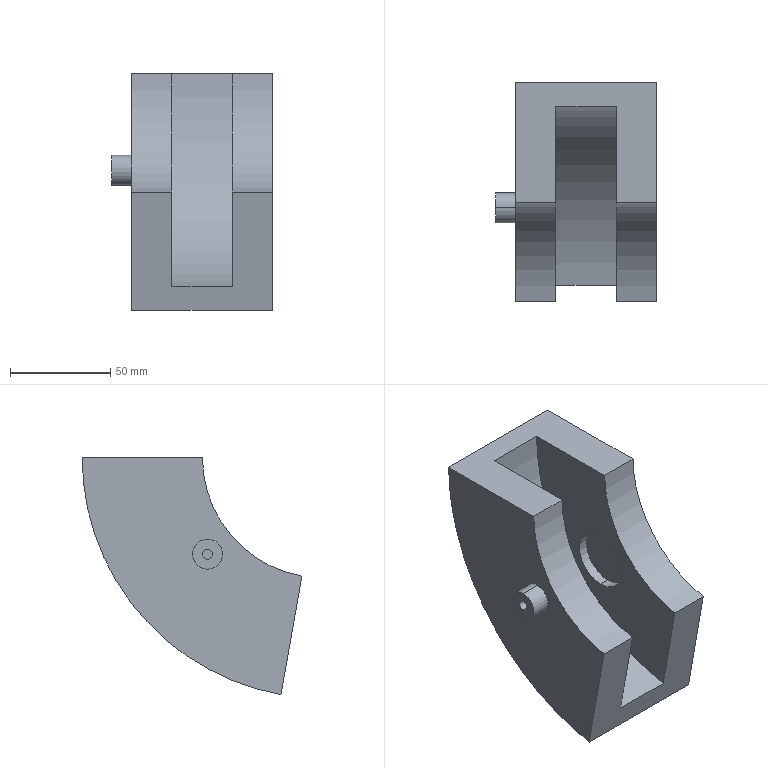Part | SolidWorks | features Cut 1, ICE 1, Revolution 1, Shell 1 | 1 solid | 29 faces | box 80 x 109.581 x 118.177 mm | volume 225708 mm3 | cylinder 16 | plane 13 | commonest cylinder face diameters 30 x4 5 x2 15 x2 120 x2 130 x2 216 x1
STEP:
#1=CARTESIAN_POINT('',(-35.136,61.532,-67.709));
#2=VERTEX_POINT('',#1);
#3=CARTESIAN_POINT('',(-35.136,61.532,-37.709));
#4=VERTEX_POINT('',#3);
#5=CARTESIAN_POINT('',(-35.136,61.532,-52.709));
#6=DIRECTION('',(-1.,0.,0.));
#7=DIRECTION('',(0.,1.,0.));
#8=AXIS2_PLACEMENT_3D('',#5,#6,#7);
#9=CIRCLE('',#8,15.);
#10=EDGE_CURVE('',#2,#4,#9,.T.);
#11=ORIENTED_EDGE('',*,*,#10,.T.);
#12=CARTESIAN_POINT('',(-30.136,61.532,-37.709));
#13=VERTEX_POINT('',#12);
#14=CARTESIAN_POINT('',(-60.137,61.532,-37.709));
#15=DIRECTION('',(1.,0.,0.));
#16=VECTOR('',#15,1000.);
#17=LINE('',#14,#16);
#18=EDGE_CURVE('',#4,#13,#17,.T.);
#19=ORIENTED_EDGE('',*,*,#18,.T.);
#20=CARTESIAN_POINT('',(-30.136,61.532,-67.709));
#21=VERTEX_POINT('',#20);
#22=CARTESIAN_POINT('',(-30.136,61.532,-52.709));
#23=DIRECTION('',(1.,0.,0.));
#24=DIRECTION('',(0.,0.,-1.));
#25=AXIS2_PLACEMENT_3D('',#22,#23,#24);
#26=CIRCLE('',#25,15.);
#27=EDGE_CURVE('',#13,#21,#26,.T.);
#28=ORIENTED_EDGE('',*,*,#27,.T.);
#29=CARTESIAN_POINT('',(-60.137,61.532,-67.709));
#30=DIRECTION('',(1.,0.,0.));
#31=VECTOR('',#30,1000.);
#32=LINE('',#29,#31);
#33=EDGE_CURVE('',#2,#21,#32,.T.);
#34=ORIENTED_EDGE('',*,*,#33,.F.);
#35=EDGE_LOOP('',(#11,#19,#28,#34));
#36=FACE_OUTER_BOUND('',#35,.T.);
#37=CARTESIAN_POINT('',(-60.137,61.532,-52.709));
#38=DIRECTION('',(1.,0.,0.));
#39=DIRECTION('',(0.,0.,-1.));
#40=AXIS2_PLACEMENT_3D('',#37,#38,#39);
#41=CYLINDRICAL_SURFACE('',#40,15.);
#42=ADVANCED_FACE('',(#36),#41,.F.);
#43=CARTESIAN_POINT('',(4.864,61.532,-67.709));
#44=VERTEX_POINT('',#43);
#45=CARTESIAN_POINT('',(4.864,61.532,-37.709));
#46=VERTEX_POINT('',#45);
#47=CARTESIAN_POINT('',(4.864,61.532,-52.709));
#48=DIRECTION('',(-1.,0.,0.));
#49=DIRECTION('',(0.,-1.,0.));
#50=AXIS2_PLACEMENT_3D('',#47,#48,#49);
#51=CIRCLE('',#50,15.);
#52=EDGE_CURVE('',#44,#46,#51,.T.);
#53=ORIENTED_EDGE('',*,*,#52,.F.);
#54=CARTESIAN_POINT('',(-0.1364,61.532,-67.709));
#55=VERTEX_POINT('',#54);
#56=CARTESIAN_POINT('',(19.865,61.532,-67.709));
#57=DIRECTION('',(-1.,0.,0.));
#58=VECTOR('',#57,1000.);
#59=LINE('',#56,#58);
#60=EDGE_CURVE('',#44,#55,#59,.T.);
#61=ORIENTED_EDGE('',*,*,#60,.T.);
#62=CARTESIAN_POINT('',(-0.1364,61.532,-37.709));
#63=VERTEX_POINT('',#62);
#64=CARTESIAN_POINT('',(-0.1364,61.532,-52.709));
#65=DIRECTION('',(-1.,0.,0.));
#66=DIRECTION('',(0.,-1.,0.));
#67=AXIS2_PLACEMENT_3D('',#64,#65,#66);
#68=CIRCLE('',#67,15.);
#69=EDGE_CURVE('',#55,#63,#68,.T.);
#70=ORIENTED_EDGE('',*,*,#69,.T.);
#71=CARTESIAN_POINT('',(19.865,61.532,-37.709));
#72=DIRECTION('',(-1.,0.,0.));
#73=VECTOR('',#72,1000.);
#74=LINE('',#71,#73);
#75=EDGE_CURVE('',#46,#63,#74,.T.);
#76=ORIENTED_EDGE('',*,*,#75,.F.);
#77=EDGE_LOOP('',(#53,#61,#70,#76));
#78=FACE_OUTER_BOUND('',#77,.T.);
#79=CARTESIAN_POINT('',(19.865,61.532,-52.709));
#80=DIRECTION('',(-1.,0.,0.));
#81=DIRECTION('',(0.,0.,1.));
#82=AXIS2_PLACEMENT_3D('',#79,#80,#81);
#83=CYLINDRICAL_SURFACE('',#82,15.);
#84=ADVANCED_FACE('',(#78),#83,.F.);
#85=CARTESIAN_POINT('',(-60.136,56.17,-50.709));
#86=VERTEX_POINT('',#85);
#87=CARTESIAN_POINT('',(-60.136,56.17,-45.709));
#88=VERTEX_POINT('',#87);
#89=CARTESIAN_POINT('',(-60.136,56.17,-48.209));
#90=DIRECTION('',(-1.,0.,0.));
#91=DIRECTION('',(0.,0.,1.));
#92=AXIS2_PLACEMENT_3D('',#89,#90,#91);
#93=CIRCLE('',#92,2.5);
#94=EDGE_CURVE('',#86,#88,#93,.T.);
#95=ORIENTED_EDGE('',*,*,#94,.T.);
#96=CARTESIAN_POINT('',(-45.136,56.17,-45.709));
#97=VERTEX_POINT('',#96);
#98=CARTESIAN_POINT('',(-60.136,56.17,-45.709));
#99=DIRECTION('',(1.,0.,0.));
#100=VECTOR('',#99,1000.);
#101=LINE('',#98,#100);
#102=EDGE_CURVE('',#88,#97,#101,.T.);
#103=ORIENTED_EDGE('',*,*,#102,.T.);
#104=CARTESIAN_POINT('',(-45.136,56.17,-50.709));
#105=VERTEX_POINT('',#104);
#106=CARTESIAN_POINT('',(-45.136,56.17,-48.209));
#107=DIRECTION('',(-1.,0.,0.));
#108=DIRECTION('',(0.,-1.,0.));
#109=AXIS2_PLACEMENT_3D('',#106,#107,#108);
#110=CIRCLE('',#109,2.5);
#111=EDGE_CURVE('',#105,#97,#110,.T.);
#112=ORIENTED_EDGE('',*,*,#111,.F.);
#113=CARTESIAN_POINT('',(-60.136,56.17,-50.709));
#114=DIRECTION('',(1.,0.,0.));
#115=VECTOR('',#114,1000.);
#116=LINE('',#113,#115);
#117=EDGE_CURVE('',#86,#105,#116,.T.);
#118=ORIENTED_EDGE('',*,*,#117,.F.);
#119=EDGE_LOOP('',(#95,#103,#112,#118));
#120=FACE_OUTER_BOUND('',#119,.T.);
#121=CARTESIAN_POINT('',(-60.136,56.17,-48.209));
#122=DIRECTION('',(1.,0.,0.));
#123=DIRECTION('',(0.,0.,-1.));
#124=AXIS2_PLACEMENT_3D('',#121,#122,#123);
#125=CYLINDRICAL_SURFACE('',#124,2.5);
#126=ADVANCED_FACE('',(#120),#125,.F.);
#127=CARTESIAN_POINT('',(-60.136,56.17,-40.709));
#128=VERTEX_POINT('',#127);
#129=CARTESIAN_POINT('',(-60.136,56.17,-55.709));
#130=VERTEX_POINT('',#129);
#131=CARTESIAN_POINT('',(-60.136,56.17,-48.209));
#132=DIRECTION('',(-1.,0.,0.));
#133=DIRECTION('',(0.,0.,1.));
#134=AXIS2_PLACEMENT_3D('',#131,#132,#133);
#135=CIRCLE('',#134,7.5);
#136=EDGE_CURVE('',#128,#130,#135,.T.);
#137=ORIENTED_EDGE('',*,*,#136,.F.);
#138=CARTESIAN_POINT('',(-50.136,56.17,-40.709));
#139=VERTEX_POINT('',#138);
#140=CARTESIAN_POINT('',(-60.136,56.17,-40.709));
#141=DIRECTION('',(1.,0.,0.));
#142=VECTOR('',#141,1000.);
#143=LINE('',#140,#142);
#144=EDGE_CURVE('',#128,#139,#143,.T.);
#145=ORIENTED_EDGE('',*,*,#144,.T.);
#146=CARTESIAN_POINT('',(-50.136,56.17,-55.709));
#147=VERTEX_POINT('',#146);
#148=CARTESIAN_POINT('',(-50.136,56.17,-48.209));
#149=DIRECTION('',(-1.,0.,0.));
#150=DIRECTION('',(0.,0.,1.));
#151=AXIS2_PLACEMENT_3D('',#148,#149,#150);
#152=CIRCLE('',#151,7.5);
#153=EDGE_CURVE('',#139,#147,#152,.T.);
#154=ORIENTED_EDGE('',*,*,#153,.T.);
#155=CARTESIAN_POINT('',(-60.136,56.17,-55.709));
#156=DIRECTION('',(1.,0.,0.));
#157=VECTOR('',#156,1000.);
#158=LINE('',#155,#157);
#159=EDGE_CURVE('',#130,#147,#158,.T.);
#160=ORIENTED_EDGE('',*,*,#159,.F.);
#161=EDGE_LOOP('',(#137,#145,#154,#160));
#162=FACE_OUTER_BOUND('',#161,.T.);
#163=CARTESIAN_POINT('',(-60.136,56.17,-48.209));
#164=DIRECTION('',(1.,0.,0.));
#165=DIRECTION('',(0.,0.,-1.));
#166=AXIS2_PLACEMENT_3D('',#163,#164,#165);
#167=CYLINDRICAL_SURFACE('',#166,7.5);
#168=ADVANCED_FACE('',(#162),#167,.T.);
#169=CARTESIAN_POINT('',(-0.1364,9.135,-59.088));
#170=VERTEX_POINT('',#169);
#171=CARTESIAN_POINT('',(-0.1364,58.717,0.));
#172=VERTEX_POINT('',#171);
#173=CARTESIAN_POINT('',(-0.1364,-1.283,0.));
#174=DIRECTION('',(1.,0.,0.));
#175=DIRECTION('',(0.,1.,0.));
#176=AXIS2_PLACEMENT_3D('',#173,#174,#175);
#177=CIRCLE('',#176,60.);
#178=EDGE_CURVE('',#170,#172,#177,.T.);
#179=ORIENTED_EDGE('',*,*,#178,.T.);
#180=CARTESIAN_POINT('',(-0.1364,106.717,0.));
#181=VERTEX_POINT('',#180);
#182=CARTESIAN_POINT('',(-0.1364,58.717,0.));
#183=DIRECTION('',(0.,-1.,0.));
#184=VECTOR('',#183,1000.);
#185=LINE('',#182,#184);
#186=EDGE_CURVE('',#181,#172,#185,.T.);
#187=ORIENTED_EDGE('',*,*,#186,.F.);
#188=CARTESIAN_POINT('',(-0.1364,17.471,-106.359));
#189=VERTEX_POINT('',#188);
#190=CARTESIAN_POINT('',(-0.1364,-1.283,0.));
#191=DIRECTION('',(1.,0.,0.));
#192=DIRECTION('',(0.,1.,0.));
#193=AXIS2_PLACEMENT_3D('',#190,#191,#192);
#194=CIRCLE('',#193,108.);
#195=EDGE_CURVE('',#189,#181,#194,.T.);
#196=ORIENTED_EDGE('',*,*,#195,.F.);
#197=CARTESIAN_POINT('',(-0.1364,9.135,-59.088));
#198=DIRECTION('',(0.,-0.1736,0.9848));
#199=VECTOR('',#198,1000.);
#200=LINE('',#197,#199);
#201=EDGE_CURVE('',#189,#170,#200,.T.);
#202=ORIENTED_EDGE('',*,*,#201,.T.);
#203=EDGE_LOOP('',(#179,#187,#196,#202));
#204=FACE_OUTER_BOUND('',#203,.T.);
#205=CARTESIAN_POINT('',(-0.1364,61.532,-52.709));
#206=DIRECTION('',(-1.,0.,0.));
#207=DIRECTION('',(0.,-1.,0.));
#208=AXIS2_PLACEMENT_3D('',#205,#206,#207);
#209=CIRCLE('',#208,15.);
#210=EDGE_CURVE('',#63,#55,#209,.T.);
#211=ORIENTED_EDGE('',*,*,#210,.F.);
#212=ORIENTED_EDGE('',*,*,#69,.F.);
#213=EDGE_LOOP('',(#211,#212));
#214=FACE_BOUND('',#213,.T.);
#215=CARTESIAN_POINT('',(-0.1364,9.135,-59.088));
#216=DIRECTION('',(-1.,0.,0.));
#217=DIRECTION('',(0.,-1.,0.));
#218=AXIS2_PLACEMENT_3D('',#215,#216,#217);
#219=PLANE('',#218);
#220=ADVANCED_FACE('',(#204,#214),#219,.T.);
#221=CARTESIAN_POINT('',(4.864,14.894,-62.955));
#222=VERTEX_POINT('',#221);
#223=CARTESIAN_POINT('',(4.864,63.524,-5.));
#224=VERTEX_POINT('',#223);
#225=CARTESIAN_POINT('',(4.864,-1.283,0.));
#226=DIRECTION('',(1.,0.,0.));
#227=DIRECTION('',(0.,-1.,0.));
#228=AXIS2_PLACEMENT_3D('',#225,#226,#227);
#229=CIRCLE('',#228,65.);
#230=EDGE_CURVE('',#222,#224,#229,.T.);
#231=ORIENTED_EDGE('',*,*,#230,.F.);
#232=CARTESIAN_POINT('',(4.864,23.244,-110.306));
#233=VERTEX_POINT('',#232);
#234=CARTESIAN_POINT('',(4.864,3.863,-0.3957));
#235=DIRECTION('',(0.,-0.1736,0.9848));
#236=VECTOR('',#235,1000.);
#237=LINE('',#234,#236);
#238=EDGE_CURVE('',#233,#222,#237,.T.);
#239=ORIENTED_EDGE('',*,*,#238,.F.);
#240=CARTESIAN_POINT('',(4.864,111.606,-5.));
#241=VERTEX_POINT('',#240);
#242=CARTESIAN_POINT('',(4.864,-1.283,0.));
#243=DIRECTION('',(1.,0.,0.));
#244=DIRECTION('',(0.,-1.,0.));
#245=AXIS2_PLACEMENT_3D('',#242,#243,#244);
#246=CIRCLE('',#245,113.);
#247=EDGE_CURVE('',#233,#241,#246,.T.);
#248=ORIENTED_EDGE('',*,*,#247,.T.);
#249=CARTESIAN_POINT('',(4.864,0.,-5.));
#250=DIRECTION('',(0.,-1.,0.));
#251=VECTOR('',#250,1000.);
#252=LINE('',#249,#251);
#253=EDGE_CURVE('',#241,#224,#252,.T.);
#254=ORIENTED_EDGE('',*,*,#253,.T.);
#255=EDGE_LOOP('',(#231,#239,#248,#254));
#256=FACE_OUTER_BOUND('',#255,.T.);
#257=CARTESIAN_POINT('',(4.864,61.532,-52.709));
#258=DIRECTION('',(-1.,0.,0.));
#259=DIRECTION('',(0.,-1.,0.));
#260=AXIS2_PLACEMENT_3D('',#257,#258,#259);
#261=CIRCLE('',#260,15.);
#262=EDGE_CURVE('',#46,#44,#261,.T.);
#263=ORIENTED_EDGE('',*,*,#262,.T.);
#264=ORIENTED_EDGE('',*,*,#52,.T.);
#265=EDGE_LOOP('',(#263,#264));
#266=FACE_BOUND('',#265,.T.);
#267=CARTESIAN_POINT('',(4.864,9.135,-59.088));
#268=DIRECTION('',(-1.,0.,0.));
#269=DIRECTION('',(0.,-1.,0.));
#270=AXIS2_PLACEMENT_3D('',#267,#268,#269);
#271=PLANE('',#270);
#272=ADVANCED_FACE('',(#256,#266),#271,.F.);
#273=CARTESIAN_POINT('',(-50.136,9.135,-59.088));
#274=VERTEX_POINT('',#273);
#275=CARTESIAN_POINT('',(-50.136,58.717,0.));
#276=VERTEX_POINT('',#275);
#277=CARTESIAN_POINT('',(-50.136,-1.283,0.));
#278=DIRECTION('',(1.,0.,0.));
#279=DIRECTION('',(0.,1.,0.));
#280=AXIS2_PLACEMENT_3D('',#277,#278,#279);
#281=CIRCLE('',#280,60.);
#282=EDGE_CURVE('',#274,#276,#281,.T.);
#283=ORIENTED_EDGE('',*,*,#282,.T.);
#284=CARTESIAN_POINT('',(-50.136,118.717,0.));
#285=VERTEX_POINT('',#284);
#286=CARTESIAN_POINT('',(-50.136,58.717,0.));
#287=DIRECTION('',(0.,-1.,0.));
#288=VECTOR('',#287,1000.);
#289=LINE('',#286,#288);
#290=EDGE_CURVE('',#285,#276,#289,.T.);
#291=ORIENTED_EDGE('',*,*,#290,.F.);
#292=CARTESIAN_POINT('',(-50.136,19.554,-118.177));
#293=VERTEX_POINT('',#292);
#294=CARTESIAN_POINT('',(-50.136,-1.283,0.));
#295=DIRECTION('',(1.,0.,0.));
#296=DIRECTION('',(0.,1.,0.));
#297=AXIS2_PLACEMENT_3D('',#294,#295,#296);
#298=CIRCLE('',#297,120.);
#299=EDGE_CURVE('',#293,#285,#298,.T.);
#300=ORIENTED_EDGE('',*,*,#299,.F.);
#301=CARTESIAN_POINT('',(-50.136,9.135,-59.088));
#302=DIRECTION('',(0.,-0.1736,0.9848));
#303=VECTOR('',#302,1000.);
#304=LINE('',#301,#303);
#305=EDGE_CURVE('',#293,#274,#304,.T.);
#306=ORIENTED_EDGE('',*,*,#305,.T.);
#307=EDGE_LOOP('',(#283,#291,#300,#306));
#308=FACE_OUTER_BOUND('',#307,.T.);
#309=CARTESIAN_POINT('',(-50.136,56.17,-48.209));
#310=DIRECTION('',(-1.,0.,0.));
#311=DIRECTION('',(0.,0.,1.));
#312=AXIS2_PLACEMENT_3D('',#309,#310,#311);
#313=CIRCLE('',#312,7.5);
#314=EDGE_CURVE('',#147,#139,#313,.T.);
#315=ORIENTED_EDGE('',*,*,#314,.F.);
#316=ORIENTED_EDGE('',*,*,#153,.F.);
#317=EDGE_LOOP('',(#315,#316));
#318=FACE_BOUND('',#317,.T.);
#319=CARTESIAN_POINT('',(-50.136,9.135,-59.088));
#320=DIRECTION('',(-1.,0.,0.));
#321=DIRECTION('',(0.,-1.,0.));
#322=AXIS2_PLACEMENT_3D('',#319,#320,#321);
#323=PLANE('',#322);
#324=ADVANCED_FACE('',(#308,#318),#323,.T.);
#325=CARTESIAN_POINT('',(19.864,9.135,-59.088));
#326=VERTEX_POINT('',#325);
#327=CARTESIAN_POINT('',(19.864,58.717,0.));
#328=VERTEX_POINT('',#327);
#329=CARTESIAN_POINT('',(19.864,-1.283,0.));
#330=DIRECTION('',(1.,0.,0.));
#331=DIRECTION('',(0.,1.,0.));
#332=AXIS2_PLACEMENT_3D('',#329,#330,#331);
#333=CIRCLE('',#332,60.);
#334=EDGE_CURVE('',#326,#328,#333,.T.);
#335=ORIENTED_EDGE('',*,*,#334,.T.);
#336=CARTESIAN_POINT('',(-0.1364,58.717,0.));
#337=DIRECTION('',(1.,0.,0.));
#338=VECTOR('',#337,1000.);
#339=LINE('',#336,#338);
#340=EDGE_CURVE('',#172,#328,#339,.T.);
#341=ORIENTED_EDGE('',*,*,#340,.F.);
#342=ORIENTED_EDGE('',*,*,#178,.F.);
#343=CARTESIAN_POINT('',(-0.1364,9.135,-59.088));
#344=DIRECTION('',(1.,0.,0.));
#345=VECTOR('',#344,1000.);
#346=LINE('',#343,#345);
#347=EDGE_CURVE('',#170,#326,#346,.T.);
#348=ORIENTED_EDGE('',*,*,#347,.T.);
#349=EDGE_LOOP('',(#335,#341,#342,#348));
#350=FACE_OUTER_BOUND('',#349,.T.);
#351=CARTESIAN_POINT('',(39.541,-1.283,0.));
#352=DIRECTION('',(1.,0.,0.));
#353=DIRECTION('',(0.,1.,0.));
#354=AXIS2_PLACEMENT_3D('',#351,#352,#353);
#355=CYLINDRICAL_SURFACE('',#354,60.);
#356=ADVANCED_FACE('',(#350),#355,.F.);
#357=CARTESIAN_POINT('',(19.864,19.554,-118.177));
#358=VERTEX_POINT('',#357);
#359=CARTESIAN_POINT('',(19.864,118.717,0.));
#360=VERTEX_POINT('',#359);
#361=CARTESIAN_POINT('',(19.864,-1.283,0.));
#362=DIRECTION('',(1.,0.,0.));
#363=DIRECTION('',(0.,1.,0.));
#364=AXIS2_PLACEMENT_3D('',#361,#362,#363);
#365=CIRCLE('',#364,120.);
#366=EDGE_CURVE('',#358,#360,#365,.T.);
#367=ORIENTED_EDGE('',*,*,#366,.T.);
#368=CARTESIAN_POINT('',(19.864,58.717,0.));
#369=DIRECTION('',(0.,1.,0.));
#370=VECTOR('',#369,1000.);
#371=LINE('',#368,#370);
#372=EDGE_CURVE('',#328,#360,#371,.T.);
#373=ORIENTED_EDGE('',*,*,#372,.F.);
#374=ORIENTED_EDGE('',*,*,#334,.F.);
#375=CARTESIAN_POINT('',(19.864,9.135,-59.088));
#376=DIRECTION('',(0.,0.1736,-0.9848));
#377=VECTOR('',#376,1000.);
#378=LINE('',#375,#377);
#379=EDGE_CURVE('',#326,#358,#378,.T.);
#380=ORIENTED_EDGE('',*,*,#379,.T.);
#381=EDGE_LOOP('',(#367,#373,#374,#380));
#382=FACE_OUTER_BOUND('',#381,.T.);
#383=CARTESIAN_POINT('',(19.864,9.135,-59.088));
#384=DIRECTION('',(1.,0.,0.));
#385=DIRECTION('',(0.,1.,0.));
#386=AXIS2_PLACEMENT_3D('',#383,#384,#385);
#387=PLANE('',#386);
#388=ADVANCED_FACE('',(#382),#387,.T.);
#389=ORIENTED_EDGE('',*,*,#299,.T.);
#390=CARTESIAN_POINT('',(-50.136,118.717,0.));
#391=DIRECTION('',(-1.,0.,0.));
#392=VECTOR('',#391,1000.);
#393=LINE('',#390,#392);
#394=EDGE_CURVE('',#360,#285,#393,.T.);
#395=ORIENTED_EDGE('',*,*,#394,.F.);
#396=ORIENTED_EDGE('',*,*,#366,.F.);
#397=CARTESIAN_POINT('',(-50.136,19.554,-118.177));
#398=DIRECTION('',(-1.,0.,0.));
#399=VECTOR('',#398,1000.);
#400=LINE('',#397,#399);
#401=EDGE_CURVE('',#358,#293,#400,.T.);
#402=ORIENTED_EDGE('',*,*,#401,.T.);
#403=EDGE_LOOP('',(#389,#395,#396,#402));
#404=FACE_OUTER_BOUND('',#403,.T.);
#405=CARTESIAN_POINT('',(39.541,-1.283,0.));
#406=DIRECTION('',(1.,0.,0.));
#407=DIRECTION('',(0.,1.,0.));
#408=AXIS2_PLACEMENT_3D('',#405,#406,#407);
#409=CYLINDRICAL_SURFACE('',#408,120.);
#410=ADVANCED_FACE('',(#404),#409,.T.);
#411=CARTESIAN_POINT('',(-30.136,9.135,-59.088));
#412=VERTEX_POINT('',#411);
#413=CARTESIAN_POINT('',(-30.136,58.717,0.));
#414=VERTEX_POINT('',#413);
#415=CARTESIAN_POINT('',(-30.136,-1.283,0.));
#416=DIRECTION('',(1.,0.,0.));
#417=DIRECTION('',(0.,1.,0.));
#418=AXIS2_PLACEMENT_3D('',#415,#416,#417);
#419=CIRCLE('',#418,60.);
#420=EDGE_CURVE('',#412,#414,#419,.T.);
#421=ORIENTED_EDGE('',*,*,#420,.T.);
#422=CARTESIAN_POINT('',(-30.136,58.717,0.));
#423=DIRECTION('',(1.,0.,0.));
#424=VECTOR('',#423,1000.);
#425=LINE('',#422,#424);
#426=EDGE_CURVE('',#276,#414,#425,.T.);
#427=ORIENTED_EDGE('',*,*,#426,.F.);
#428=ORIENTED_EDGE('',*,*,#282,.F.);
#429=CARTESIAN_POINT('',(-30.136,9.135,-59.088));
#430=DIRECTION('',(1.,0.,0.));
#431=VECTOR('',#430,1000.);
#432=LINE('',#429,#431);
#433=EDGE_CURVE('',#274,#412,#432,.T.);
#434=ORIENTED_EDGE('',*,*,#433,.T.);
#435=EDGE_LOOP('',(#421,#427,#428,#434));
#436=FACE_OUTER_BOUND('',#435,.T.);
#437=CARTESIAN_POINT('',(39.541,-1.283,0.));
#438=DIRECTION('',(1.,0.,0.));
#439=DIRECTION('',(0.,1.,0.));
#440=AXIS2_PLACEMENT_3D('',#437,#438,#439);
#441=CYLINDRICAL_SURFACE('',#440,60.);
#442=ADVANCED_FACE('',(#436),#441,.F.);
#443=CARTESIAN_POINT('',(-30.136,61.532,-52.709));
#444=DIRECTION('',(1.,0.,0.));
#445=DIRECTION('',(0.,0.,-1.));
#446=AXIS2_PLACEMENT_3D('',#443,#444,#445);
#447=CIRCLE('',#446,15.);
#448=EDGE_CURVE('',#21,#13,#447,.T.);
#449=ORIENTED_EDGE('',*,*,#448,.F.);
#450=ORIENTED_EDGE('',*,*,#27,.F.);
#451=EDGE_LOOP('',(#449,#450));
#452=FACE_BOUND('',#451,.T.);
#453=CARTESIAN_POINT('',(-30.136,17.471,-106.359));
#454=VERTEX_POINT('',#453);
#455=CARTESIAN_POINT('',(-30.136,106.717,0.));
#456=VERTEX_POINT('',#455);
#457=CARTESIAN_POINT('',(-30.136,-1.283,0.));
#458=DIRECTION('',(1.,0.,0.));
#459=DIRECTION('',(0.,1.,0.));
#460=AXIS2_PLACEMENT_3D('',#457,#458,#459);
#461=CIRCLE('',#460,108.);
#462=EDGE_CURVE('',#454,#456,#461,.T.);
#463=ORIENTED_EDGE('',*,*,#462,.T.);
#464=CARTESIAN_POINT('',(-30.136,106.717,0.));
#465=DIRECTION('',(0.,1.,0.));
#466=VECTOR('',#465,1000.);
#467=LINE('',#464,#466);
#468=EDGE_CURVE('',#414,#456,#467,.T.);
#469=ORIENTED_EDGE('',*,*,#468,.F.);
#470=ORIENTED_EDGE('',*,*,#420,.F.);
#471=CARTESIAN_POINT('',(-30.136,17.471,-106.359));
#472=DIRECTION('',(0.,0.1736,-0.9848));
#473=VECTOR('',#472,1000.);
#474=LINE('',#471,#473);
#475=EDGE_CURVE('',#412,#454,#474,.T.);
#476=ORIENTED_EDGE('',*,*,#475,.T.);
#477=EDGE_LOOP('',(#463,#469,#470,#476));
#478=FACE_OUTER_BOUND('',#477,.T.);
#479=CARTESIAN_POINT('',(-30.136,17.471,-106.359));
#480=DIRECTION('',(1.,0.,0.));
#481=DIRECTION('',(0.,1.,0.));
#482=AXIS2_PLACEMENT_3D('',#479,#480,#481);
#483=PLANE('',#482);
#484=ADVANCED_FACE('',(#452,#478),#483,.T.);
#485=CARTESIAN_POINT('',(-0.1364,17.471,-106.359));
#486=DIRECTION('',(1.,0.,0.));
#487=VECTOR('',#486,1000.);
#488=LINE('',#485,#487);
#489=EDGE_CURVE('',#454,#189,#488,.T.);
#490=ORIENTED_EDGE('',*,*,#489,.T.);
#491=ORIENTED_EDGE('',*,*,#195,.T.);
#492=CARTESIAN_POINT('',(-0.1364,106.717,0.));
#493=DIRECTION('',(1.,0.,0.));
#494=VECTOR('',#493,1000.);
#495=LINE('',#492,#494);
#496=EDGE_CURVE('',#456,#181,#495,.T.);
#497=ORIENTED_EDGE('',*,*,#496,.F.);
#498=ORIENTED_EDGE('',*,*,#462,.F.);
#499=EDGE_LOOP('',(#490,#491,#497,#498));
#500=FACE_OUTER_BOUND('',#499,.T.);
#501=CARTESIAN_POINT('',(39.541,-1.283,0.));
#502=DIRECTION('',(1.,0.,0.));
#503=DIRECTION('',(0.,1.,0.));
#504=AXIS2_PLACEMENT_3D('',#501,#502,#503);
#505=CYLINDRICAL_SURFACE('',#504,108.);
#506=ADVANCED_FACE('',(#500),#505,.F.);
#507=ORIENTED_EDGE('',*,*,#201,.F.);
#508=ORIENTED_EDGE('',*,*,#489,.F.);
#509=ORIENTED_EDGE('',*,*,#475,.F.);
#510=ORIENTED_EDGE('',*,*,#433,.F.);
#511=ORIENTED_EDGE('',*,*,#305,.F.);
#512=ORIENTED_EDGE('',*,*,#401,.F.);
#513=ORIENTED_EDGE('',*,*,#379,.F.);
#514=ORIENTED_EDGE('',*,*,#347,.F.);
#515=EDGE_LOOP('',(#507,#508,#509,#510,#511,#512,#513,#514));
#516=FACE_OUTER_BOUND('',#515,.T.);
#517=CARTESIAN_POINT('',(0.,-1.061,-1.264));
#518=DIRECTION('',(0.,0.9848,0.1736));
#519=DIRECTION('',(1.,0.,0.));
#520=AXIS2_PLACEMENT_3D('',#517,#518,#519);
#521=PLANE('',#520);
#522=ADVANCED_FACE('',(#516),#521,.F.);
#523=ORIENTED_EDGE('',*,*,#186,.T.);
#524=ORIENTED_EDGE('',*,*,#340,.T.);
#525=ORIENTED_EDGE('',*,*,#372,.T.);
#526=ORIENTED_EDGE('',*,*,#394,.T.);
#527=ORIENTED_EDGE('',*,*,#290,.T.);
#528=ORIENTED_EDGE('',*,*,#426,.T.);
#529=ORIENTED_EDGE('',*,*,#468,.T.);
#530=ORIENTED_EDGE('',*,*,#496,.T.);
#531=EDGE_LOOP('',(#523,#524,#525,#526,#527,#528,#529,#530));
#532=FACE_OUTER_BOUND('',#531,.T.);
#533=CARTESIAN_POINT('',(0.,0.,0.));
#534=DIRECTION('',(0.,0.,1.));
#535=DIRECTION('',(1.,0.,0.));
#536=AXIS2_PLACEMENT_3D('',#533,#534,#535);
#537=PLANE('',#536);
#538=ADVANCED_FACE('',(#532),#537,.T.);
#539=ORIENTED_EDGE('',*,*,#144,.F.);
#540=CARTESIAN_POINT('',(-60.136,56.17,-48.209));
#541=DIRECTION('',(-1.,0.,0.));
#542=DIRECTION('',(0.,0.,1.));
#543=AXIS2_PLACEMENT_3D('',#540,#541,#542);
#544=CIRCLE('',#543,7.5);
#545=EDGE_CURVE('',#130,#128,#544,.T.);
#546=ORIENTED_EDGE('',*,*,#545,.F.);
#547=ORIENTED_EDGE('',*,*,#159,.T.);
#548=ORIENTED_EDGE('',*,*,#314,.T.);
#549=EDGE_LOOP('',(#539,#546,#547,#548));
#550=FACE_OUTER_BOUND('',#549,.T.);
#551=CARTESIAN_POINT('',(-60.136,56.17,-48.209));
#552=DIRECTION('',(1.,0.,0.));
#553=DIRECTION('',(0.,0.,-1.));
#554=AXIS2_PLACEMENT_3D('',#551,#552,#553);
#555=CYLINDRICAL_SURFACE('',#554,7.5);
#556=ADVANCED_FACE('',(#550),#555,.T.);
#557=ORIENTED_EDGE('',*,*,#94,.F.);
#558=CARTESIAN_POINT('',(-60.136,56.17,-48.209));
#559=DIRECTION('',(-1.,0.,0.));
#560=DIRECTION('',(0.,0.,1.));
#561=AXIS2_PLACEMENT_3D('',#558,#559,#560);
#562=CIRCLE('',#561,2.5);
#563=EDGE_CURVE('',#88,#86,#562,.T.);
#564=ORIENTED_EDGE('',*,*,#563,.F.);
#565=EDGE_LOOP('',(#557,#564));
#566=FACE_BOUND('',#565,.T.);
#567=ORIENTED_EDGE('',*,*,#545,.T.);
#568=ORIENTED_EDGE('',*,*,#136,.T.);
#569=EDGE_LOOP('',(#567,#568));
#570=FACE_OUTER_BOUND('',#569,.T.);
#571=CARTESIAN_POINT('',(-60.136,56.17,-48.209));
#572=DIRECTION('',(-1.,0.,0.));
#573=DIRECTION('',(0.,0.,1.));
#574=AXIS2_PLACEMENT_3D('',#571,#572,#573);
#575=PLANE('',#574);
#576=ADVANCED_FACE('',(#566,#570),#575,.T.);
#577=CARTESIAN_POINT('',(-45.136,14.894,-62.955));
#578=VERTEX_POINT('',#577);
#579=CARTESIAN_POINT('',(-45.136,63.524,-5.));
#580=VERTEX_POINT('',#579);
#581=CARTESIAN_POINT('',(-45.136,-1.283,0.));
#582=DIRECTION('',(1.,0.,0.));
#583=DIRECTION('',(0.,-1.,0.));
#584=AXIS2_PLACEMENT_3D('',#581,#582,#583);
#585=CIRCLE('',#584,65.);
#586=EDGE_CURVE('',#578,#580,#585,.T.);
#587=ORIENTED_EDGE('',*,*,#586,.F.);
#588=CARTESIAN_POINT('',(-45.136,23.591,-112.278));
#589=VERTEX_POINT('',#588);
#590=CARTESIAN_POINT('',(-45.136,3.863,-0.3957));
#591=DIRECTION('',(0.,-0.1736,0.9848));
#592=VECTOR('',#591,1000.);
#593=LINE('',#590,#592);
#594=EDGE_CURVE('',#589,#578,#593,.T.);
#595=ORIENTED_EDGE('',*,*,#594,.F.);
#596=CARTESIAN_POINT('',(-45.136,113.608,-5.));
#597=VERTEX_POINT('',#596);
#598=CARTESIAN_POINT('',(-45.136,-1.283,0.));
#599=DIRECTION('',(1.,0.,0.));
#600=DIRECTION('',(0.,-1.,0.));
#601=AXIS2_PLACEMENT_3D('',#598,#599,#600);
#602=CIRCLE('',#601,115.);
#603=EDGE_CURVE('',#589,#597,#602,.T.);
#604=ORIENTED_EDGE('',*,*,#603,.T.);
#605=CARTESIAN_POINT('',(-45.136,0.,-5.));
#606=DIRECTION('',(0.,-1.,0.));
#607=VECTOR('',#606,1000.);
#608=LINE('',#605,#607);
#609=EDGE_CURVE('',#597,#580,#608,.T.);
#610=ORIENTED_EDGE('',*,*,#609,.T.);
#611=EDGE_LOOP('',(#587,#595,#604,#610));
#612=FACE_OUTER_BOUND('',#611,.T.);
#613=ORIENTED_EDGE('',*,*,#111,.T.);
#614=CARTESIAN_POINT('',(-45.136,56.17,-48.209));
#615=DIRECTION('',(-1.,0.,0.));
#616=DIRECTION('',(0.,-1.,0.));
#617=AXIS2_PLACEMENT_3D('',#614,#615,#616);
#618=CIRCLE('',#617,2.5);
#619=EDGE_CURVE('',#97,#105,#618,.T.);
#620=ORIENTED_EDGE('',*,*,#619,.T.);
#621=EDGE_LOOP('',(#613,#620));
#622=FACE_BOUND('',#621,.T.);
#623=CARTESIAN_POINT('',(-45.136,9.135,-59.088));
#624=DIRECTION('',(-1.,0.,0.));
#625=DIRECTION('',(0.,-1.,0.));
#626=AXIS2_PLACEMENT_3D('',#623,#624,#625);
#627=PLANE('',#626);
#628=ADVANCED_FACE('',(#612,#622),#627,.F.);
#629=CARTESIAN_POINT('',(14.864,14.894,-62.955));
#630=VERTEX_POINT('',#629);
#631=CARTESIAN_POINT('',(14.864,63.524,-5.));
#632=VERTEX_POINT('',#631);
#633=CARTESIAN_POINT('',(14.864,-1.283,0.));
#634=DIRECTION('',(1.,0.,0.));
#635=DIRECTION('',(0.,1.,0.));
#636=AXIS2_PLACEMENT_3D('',#633,#634,#635);
#637=CIRCLE('',#636,65.);
#638=EDGE_CURVE('',#630,#632,#637,.T.);
#639=ORIENTED_EDGE('',*,*,#638,.F.);
#640=CARTESIAN_POINT('',(4.864,14.894,-62.955));
#641=DIRECTION('',(1.,0.,0.));
#642=VECTOR('',#641,1000.);
#643=LINE('',#640,#642);
#644=EDGE_CURVE('',#222,#630,#643,.T.);
#645=ORIENTED_EDGE('',*,*,#644,.F.);
#646=ORIENTED_EDGE('',*,*,#230,.T.);
#647=CARTESIAN_POINT('',(4.864,63.524,-5.));
#648=DIRECTION('',(1.,0.,0.));
#649=VECTOR('',#648,1000.);
#650=LINE('',#647,#649);
#651=EDGE_CURVE('',#224,#632,#650,.T.);
#652=ORIENTED_EDGE('',*,*,#651,.T.);
#653=EDGE_LOOP('',(#639,#645,#646,#652));
#654=FACE_OUTER_BOUND('',#653,.T.);
#655=CARTESIAN_POINT('',(39.541,-1.283,0.));
#656=DIRECTION('',(1.,0.,0.));
#657=DIRECTION('',(0.,1.,0.));
#658=AXIS2_PLACEMENT_3D('',#655,#656,#657);
#659=CYLINDRICAL_SURFACE('',#658,65.);
#660=ADVANCED_FACE('',(#654),#659,.T.);
#661=CARTESIAN_POINT('',(14.864,23.591,-112.278));
#662=VERTEX_POINT('',#661);
#663=CARTESIAN_POINT('',(14.864,113.608,-5.));
#664=VERTEX_POINT('',#663);
#665=CARTESIAN_POINT('',(14.864,-1.283,0.));
#666=DIRECTION('',(1.,0.,0.));
#667=DIRECTION('',(0.,1.,0.));
#668=AXIS2_PLACEMENT_3D('',#665,#666,#667);
#669=CIRCLE('',#668,115.);
#670=EDGE_CURVE('',#662,#664,#669,.T.);
#671=ORIENTED_EDGE('',*,*,#670,.F.);
#672=CARTESIAN_POINT('',(14.864,3.863,-0.3957));
#673=DIRECTION('',(0.,0.1736,-0.9848));
#674=VECTOR('',#673,1000.);
#675=LINE('',#672,#674);
#676=EDGE_CURVE('',#630,#662,#675,.T.);
#677=ORIENTED_EDGE('',*,*,#676,.F.);
#678=ORIENTED_EDGE('',*,*,#638,.T.);
#679=CARTESIAN_POINT('',(14.864,0.,-5.));
#680=DIRECTION('',(0.,1.,0.));
#681=VECTOR('',#680,1000.);
#682=LINE('',#679,#681);
#683=EDGE_CURVE('',#632,#664,#682,.T.);
#684=ORIENTED_EDGE('',*,*,#683,.T.);
#685=EDGE_LOOP('',(#671,#677,#678,#684));
#686=FACE_OUTER_BOUND('',#685,.T.);
#687=CARTESIAN_POINT('',(14.864,9.135,-59.088));
#688=DIRECTION('',(1.,0.,0.));
#689=DIRECTION('',(0.,1.,0.));
#690=AXIS2_PLACEMENT_3D('',#687,#688,#689);
#691=PLANE('',#690);
#692=ADVANCED_FACE('',(#686),#691,.F.);
#693=ORIENTED_EDGE('',*,*,#603,.F.);
#694=CARTESIAN_POINT('',(14.864,23.591,-112.278));
#695=DIRECTION('',(-1.,0.,0.));
#696=VECTOR('',#695,1000.);
#697=LINE('',#694,#696);
#698=EDGE_CURVE('',#662,#589,#697,.T.);
#699=ORIENTED_EDGE('',*,*,#698,.F.);
#700=ORIENTED_EDGE('',*,*,#670,.T.);
#701=CARTESIAN_POINT('',(14.864,113.608,-5.));
#702=DIRECTION('',(-1.,0.,0.));
#703=VECTOR('',#702,1000.);
#704=LINE('',#701,#703);
#705=EDGE_CURVE('',#664,#597,#704,.T.);
#706=ORIENTED_EDGE('',*,*,#705,.T.);
#707=EDGE_LOOP('',(#693,#699,#700,#706));
#708=FACE_OUTER_BOUND('',#707,.T.);
#709=CARTESIAN_POINT('',(39.541,-1.283,0.));
#710=DIRECTION('',(1.,0.,0.));
#711=DIRECTION('',(0.,1.,0.));
#712=AXIS2_PLACEMENT_3D('',#709,#710,#711);
#713=CYLINDRICAL_SURFACE('',#712,115.);
#714=ADVANCED_FACE('',(#708),#713,.F.);
#715=CARTESIAN_POINT('',(-35.136,14.894,-62.955));
#716=VERTEX_POINT('',#715);
#717=CARTESIAN_POINT('',(-35.136,63.524,-5.));
#718=VERTEX_POINT('',#717);
#719=CARTESIAN_POINT('',(-35.136,-1.283,0.));
#720=DIRECTION('',(1.,0.,0.));
#721=DIRECTION('',(0.,1.,0.));
#722=AXIS2_PLACEMENT_3D('',#719,#720,#721);
#723=CIRCLE('',#722,65.);
#724=EDGE_CURVE('',#716,#718,#723,.T.);
#725=ORIENTED_EDGE('',*,*,#724,.F.);
#726=CARTESIAN_POINT('',(-45.136,14.894,-62.955));
#727=DIRECTION('',(1.,0.,0.));
#728=VECTOR('',#727,1000.);
#729=LINE('',#726,#728);
#730=EDGE_CURVE('',#578,#716,#729,.T.);
#731=ORIENTED_EDGE('',*,*,#730,.F.);
#732=ORIENTED_EDGE('',*,*,#586,.T.);
#733=CARTESIAN_POINT('',(-45.136,63.524,-5.));
#734=DIRECTION('',(1.,0.,0.));
#735=VECTOR('',#734,1000.);
#736=LINE('',#733,#735);
#737=EDGE_CURVE('',#580,#718,#736,.T.);
#738=ORIENTED_EDGE('',*,*,#737,.T.);
#739=EDGE_LOOP('',(#725,#731,#732,#738));
#740=FACE_OUTER_BOUND('',#739,.T.);
#741=CARTESIAN_POINT('',(39.541,-1.283,0.));
#742=DIRECTION('',(1.,0.,0.));
#743=DIRECTION('',(0.,1.,0.));
#744=AXIS2_PLACEMENT_3D('',#741,#742,#743);
#745=CYLINDRICAL_SURFACE('',#744,65.);
#746=ADVANCED_FACE('',(#740),#745,.T.);
#747=ORIENTED_EDGE('',*,*,#10,.F.);
#748=CARTESIAN_POINT('',(-35.136,61.532,-52.709));
#749=DIRECTION('',(-1.,0.,0.));
#750=DIRECTION('',(0.,1.,0.));
#751=AXIS2_PLACEMENT_3D('',#748,#749,#750);
#752=CIRCLE('',#751,15.);
#753=EDGE_CURVE('',#4,#2,#752,.T.);
#754=ORIENTED_EDGE('',*,*,#753,.F.);
#755=EDGE_LOOP('',(#747,#754));
#756=FACE_BOUND('',#755,.T.);
#757=CARTESIAN_POINT('',(-35.136,23.244,-110.306));
#758=VERTEX_POINT('',#757);
#759=CARTESIAN_POINT('',(-35.136,111.606,-5.));
#760=VERTEX_POINT('',#759);
#761=CARTESIAN_POINT('',(-35.136,-1.283,0.));
#762=DIRECTION('',(1.,0.,0.));
#763=DIRECTION('',(0.,1.,0.));
#764=AXIS2_PLACEMENT_3D('',#761,#762,#763);
#765=CIRCLE('',#764,113.);
#766=EDGE_CURVE('',#758,#760,#765,.T.);
#767=ORIENTED_EDGE('',*,*,#766,.F.);
#768=CARTESIAN_POINT('',(-35.136,3.863,-0.3957));
#769=DIRECTION('',(0.,0.1736,-0.9848));
#770=VECTOR('',#769,1000.);
#771=LINE('',#768,#770);
#772=EDGE_CURVE('',#716,#758,#771,.T.);
#773=ORIENTED_EDGE('',*,*,#772,.F.);
#774=ORIENTED_EDGE('',*,*,#724,.T.);
#775=CARTESIAN_POINT('',(-35.136,0.,-5.));
#776=DIRECTION('',(0.,1.,0.));
#777=VECTOR('',#776,1000.);
#778=LINE('',#775,#777);
#779=EDGE_CURVE('',#718,#760,#778,.T.);
#780=ORIENTED_EDGE('',*,*,#779,.T.);
#781=EDGE_LOOP('',(#767,#773,#774,#780));
#782=FACE_OUTER_BOUND('',#781,.T.);
#783=CARTESIAN_POINT('',(-35.136,17.471,-106.359));
#784=DIRECTION('',(1.,0.,0.));
#785=DIRECTION('',(0.,1.,0.));
#786=AXIS2_PLACEMENT_3D('',#783,#784,#785);
#787=PLANE('',#786);
#788=ADVANCED_FACE('',(#756,#782),#787,.F.);
#789=CARTESIAN_POINT('',(-35.136,23.244,-110.306));
#790=DIRECTION('',(1.,0.,0.));
#791=VECTOR('',#790,1000.);
#792=LINE('',#789,#791);
#793=EDGE_CURVE('',#758,#233,#792,.T.);
#794=ORIENTED_EDGE('',*,*,#793,.F.);
#795=ORIENTED_EDGE('',*,*,#766,.T.);
#796=CARTESIAN_POINT('',(-35.136,111.606,-5.));
#797=DIRECTION('',(1.,0.,0.));
#798=VECTOR('',#797,1000.);
#799=LINE('',#796,#798);
#800=EDGE_CURVE('',#760,#241,#799,.T.);
#801=ORIENTED_EDGE('',*,*,#800,.T.);
#802=ORIENTED_EDGE('',*,*,#247,.F.);
#803=EDGE_LOOP('',(#794,#795,#801,#802));
#804=FACE_OUTER_BOUND('',#803,.T.);
#805=CARTESIAN_POINT('',(39.541,-1.283,0.));
#806=DIRECTION('',(1.,0.,0.));
#807=DIRECTION('',(0.,1.,0.));
#808=AXIS2_PLACEMENT_3D('',#805,#806,#807);
#809=CYLINDRICAL_SURFACE('',#808,113.);
#810=ADVANCED_FACE('',(#804),#809,.T.);
#811=ORIENTED_EDGE('',*,*,#238,.T.);
#812=ORIENTED_EDGE('',*,*,#644,.T.);
#813=ORIENTED_EDGE('',*,*,#676,.T.);
#814=ORIENTED_EDGE('',*,*,#698,.T.);
#815=ORIENTED_EDGE('',*,*,#594,.T.);
#816=ORIENTED_EDGE('',*,*,#730,.T.);
#817=ORIENTED_EDGE('',*,*,#772,.T.);
#818=ORIENTED_EDGE('',*,*,#793,.T.);
#819=EDGE_LOOP('',(#811,#812,#813,#814,#815,#816,#817,#818));
#820=FACE_OUTER_BOUND('',#819,.T.);
#821=CARTESIAN_POINT('',(0.,3.863,-0.3957));
#822=DIRECTION('',(0.,0.9848,0.1736));
#823=DIRECTION('',(1.,0.,0.));
#824=AXIS2_PLACEMENT_3D('',#821,#822,#823);
#825=PLANE('',#824);
#826=ADVANCED_FACE('',(#820),#825,.T.);
#827=ORIENTED_EDGE('',*,*,#253,.F.);
#828=ORIENTED_EDGE('',*,*,#800,.F.);
#829=ORIENTED_EDGE('',*,*,#779,.F.);
#830=ORIENTED_EDGE('',*,*,#737,.F.);
#831=ORIENTED_EDGE('',*,*,#609,.F.);
#832=ORIENTED_EDGE('',*,*,#705,.F.);
#833=ORIENTED_EDGE('',*,*,#683,.F.);
#834=ORIENTED_EDGE('',*,*,#651,.F.);
#835=EDGE_LOOP('',(#827,#828,#829,#830,#831,#832,#833,#834));
#836=FACE_OUTER_BOUND('',#835,.T.);
#837=CARTESIAN_POINT('',(0.,0.,-5.));
#838=DIRECTION('',(0.,0.,1.));
#839=DIRECTION('',(1.,0.,0.));
#840=AXIS2_PLACEMENT_3D('',#837,#838,#839);
#841=PLANE('',#840);
#842=ADVANCED_FACE('',(#836),#841,.F.);
#843=ORIENTED_EDGE('',*,*,#102,.F.);
#844=ORIENTED_EDGE('',*,*,#563,.T.);
#845=ORIENTED_EDGE('',*,*,#117,.T.);
#846=ORIENTED_EDGE('',*,*,#619,.F.);
#847=EDGE_LOOP('',(#843,#844,#845,#846));
#848=FACE_OUTER_BOUND('',#847,.T.);
#849=CARTESIAN_POINT('',(-60.136,56.17,-48.209));
#850=DIRECTION('',(1.,0.,0.));
#851=DIRECTION('',(0.,0.,-1.));
#852=AXIS2_PLACEMENT_3D('',#849,#850,#851);
#853=CYLINDRICAL_SURFACE('',#852,2.5);
#854=ADVANCED_FACE('',(#848),#853,.F.);
#855=ORIENTED_EDGE('',*,*,#60,.F.);
#856=ORIENTED_EDGE('',*,*,#262,.F.);
#857=ORIENTED_EDGE('',*,*,#75,.T.);
#858=ORIENTED_EDGE('',*,*,#210,.T.);
#859=EDGE_LOOP('',(#855,#856,#857,#858));
#860=FACE_OUTER_BOUND('',#859,.T.);
#861=CARTESIAN_POINT('',(19.865,61.532,-52.709));
#862=DIRECTION('',(-1.,0.,0.));
#863=DIRECTION('',(0.,0.,1.));
#864=AXIS2_PLACEMENT_3D('',#861,#862,#863);
#865=CYLINDRICAL_SURFACE('',#864,15.);
#866=ADVANCED_FACE('',(#860),#865,.F.);
#867=ORIENTED_EDGE('',*,*,#18,.F.);
#868=ORIENTED_EDGE('',*,*,#753,.T.);
#869=ORIENTED_EDGE('',*,*,#33,.T.);
#870=ORIENTED_EDGE('',*,*,#448,.T.);
#871=EDGE_LOOP('',(#867,#868,#869,#870));
#872=FACE_OUTER_BOUND('',#871,.T.);
#873=CARTESIAN_POINT('',(-60.137,61.532,-52.709));
#874=DIRECTION('',(1.,0.,0.));
#875=DIRECTION('',(0.,0.,-1.));
#876=AXIS2_PLACEMENT_3D('',#873,#874,#875);
#877=CYLINDRICAL_SURFACE('',#876,15.);
#878=ADVANCED_FACE('',(#872),#877,.F.);
#879=CLOSED_SHELL('',(#42,#84,#126,#168,#220,#272,#324,#356,#388,#410,#442,#484,#506,#522,#538,#556,#576,#628,#660,#692,#714,#746,#788,#810,#826,#842,#854,#866,#878));
#880=MANIFOLD_SOLID_BREP('',#879);
#881=CARTESIAN_POINT('',(0.,0.,0.));
#882=DIRECTION('',(0.,0.,1.));
#883=DIRECTION('',(1.,0.,0.));
#884=AXIS2_PLACEMENT_3D('',#881,#882,#883);
#885=(LENGTH_UNIT()NAMED_UNIT(*)SI_UNIT(.MILLI.,.METRE.));
#886=UNCERTAINTY_MEASURE_WITH_UNIT(LENGTH_MEASURE(0.00001),#885,'','');
#887=(NAMED_UNIT(*)PLANE_ANGLE_UNIT()SI_UNIT($,.RADIAN.));
#888=(NAMED_UNIT(*)SI_UNIT($,.STERADIAN.)SOLID_ANGLE_UNIT());
#889=(GEOMETRIC_REPRESENTATION_CONTEXT(3)GLOBAL_UNCERTAINTY_ASSIGNED_CONTEXT((#886))GLOBAL_UNIT_ASSIGNED_CONTEXT((#885,#887,#888))REPRESENTATION_CONTEXT('',''));
#890=ADVANCED_BREP_SHAPE_REPRESENTATION('',(#880,#884),#889);